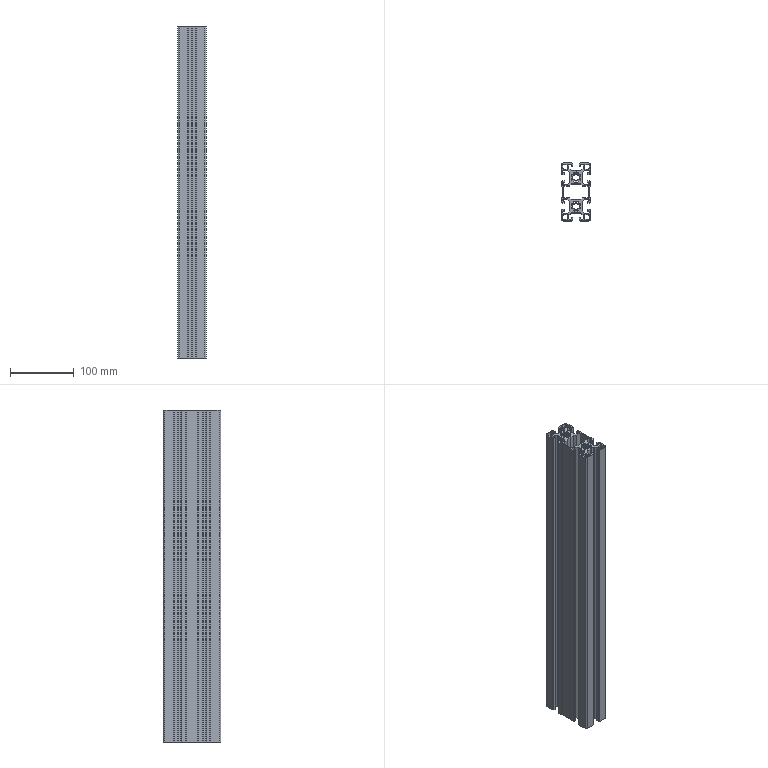Part | STEP file | PN_0006 | 1 solid | 468 faces | box 45 x 90 x 520 mm | volume 676438 mm3 | cylinder 262 | plane 206 | commonest cylinder face diameters 1 x116 0.6 x56 2 x40 10.2 x18 16 x16 0.4 x12